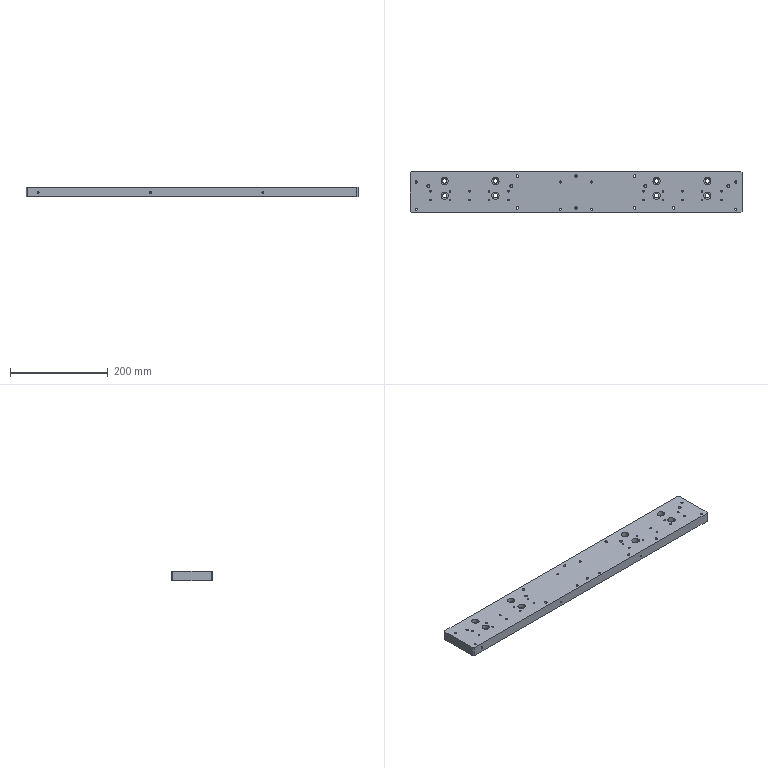Part | SolidWorks | features BaseBody 1 | 1 solid | 148 faces | box 680 x 85 x 20 mm | volume 1127691 mm3 | cylinder 116 | plane 18 | cone 14 | commonest cylinder face diameters 3.3 x46 4.2 x16 9 x16 15 x16 5 x14 6 x8